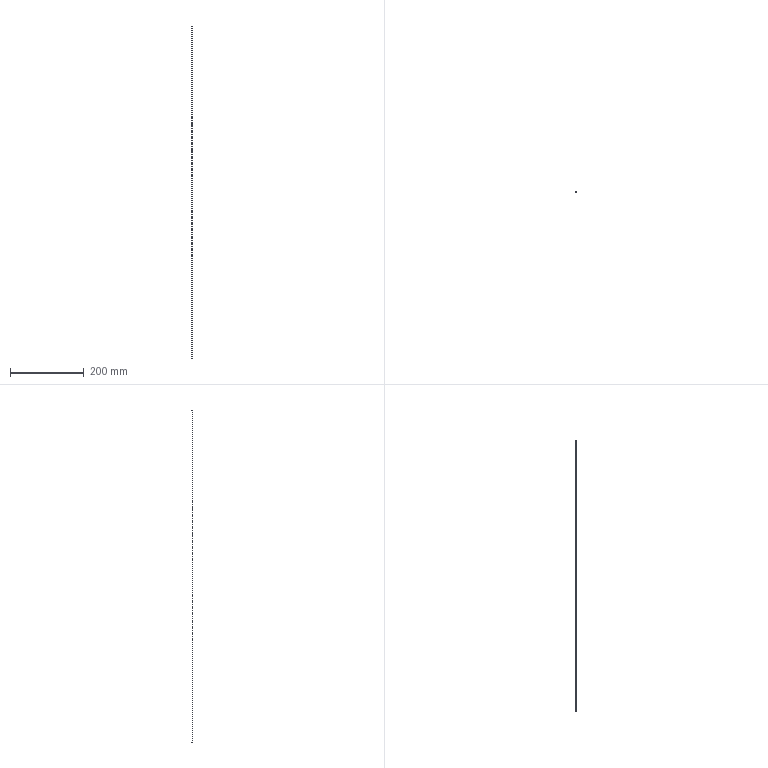Part | NX | 1 solid | 3 faces | box 2 x 2 x 900 mm | volume 2827 mm3 | plane 2 | cylinder 1 | commonest cylinder face diameters 2 x1
STEP:
#1=CARTESIAN_POINT('',(1.,0.,960.));
#2=VERTEX_POINT('',#1);
#3=CARTESIAN_POINT('',(0.,0.,960.));
#4=DIRECTION('',(0.,0.,1.));
#5=DIRECTION('',(1.,0.,0.));
#6=AXIS2_PLACEMENT_3D('',#3,#4,#5);
#7=CIRCLE('',#6,1.);
#8=EDGE_CURVE('',#2,#2,#7,.T.);
#9=ORIENTED_EDGE('',*,*,#8,.F.);
#10=EDGE_LOOP('',(#9));
#11=FACE_BOUND('',#10,.T.);
#12=CARTESIAN_POINT('',(1.,0.,60.));
#13=VERTEX_POINT('',#12);
#14=CARTESIAN_POINT('',(0.,0.,60.));
#15=DIRECTION('',(0.,0.,1.));
#16=DIRECTION('',(1.,0.,0.));
#17=AXIS2_PLACEMENT_3D('',#14,#15,#16);
#18=CIRCLE('',#17,1.);
#19=EDGE_CURVE('',#13,#13,#18,.T.);
#20=ORIENTED_EDGE('',*,*,#19,.T.);
#21=EDGE_LOOP('',(#20));
#22=FACE_BOUND('',#21,.T.);
#23=CARTESIAN_POINT('',(0.,0.,960.));
#24=DIRECTION('',(0.,0.,-1.));
#25=DIRECTION('',(-1.,0.,0.));
#26=AXIS2_PLACEMENT_3D('',#23,#24,#25);
#27=CYLINDRICAL_SURFACE('',#26,1.);
#28=ADVANCED_FACE('',(#11,#22),#27,.T.);
#29=ORIENTED_EDGE('',*,*,#8,.T.);
#30=EDGE_LOOP('',(#29));
#31=FACE_BOUND('',#30,.T.);
#32=CARTESIAN_POINT('',(0.,0.,960.));
#33=DIRECTION('',(0.,0.,1.));
#34=DIRECTION('',(1.,0.,0.));
#35=AXIS2_PLACEMENT_3D('',#32,#33,#34);
#36=PLANE('',#35);
#37=ADVANCED_FACE('',(#31),#36,.T.);
#38=ORIENTED_EDGE('',*,*,#19,.F.);
#39=EDGE_LOOP('',(#38));
#40=FACE_BOUND('',#39,.T.);
#41=CARTESIAN_POINT('',(0.,0.,60.));
#42=DIRECTION('',(0.,0.,1.));
#43=DIRECTION('',(1.,0.,0.));
#44=AXIS2_PLACEMENT_3D('',#41,#42,#43);
#45=PLANE('',#44);
#46=ADVANCED_FACE('',(#40),#45,.F.);
#47=CLOSED_SHELL('',(#28,#37,#46));
#48=MANIFOLD_SOLID_BREP('',#47);
#49=(LENGTH_UNIT()NAMED_UNIT(*)SI_UNIT(.MILLI.,.METRE.));
#50=UNCERTAINTY_MEASURE_WITH_UNIT(LENGTH_MEASURE(0.00001),#49,'','');
#51=(NAMED_UNIT(*)PLANE_ANGLE_UNIT()SI_UNIT($,.RADIAN.));
#52=(NAMED_UNIT(*)SI_UNIT($,.STERADIAN.)SOLID_ANGLE_UNIT());
#53=(GEOMETRIC_REPRESENTATION_CONTEXT(3)GLOBAL_UNCERTAINTY_ASSIGNED_CONTEXT((#50))GLOBAL_UNIT_ASSIGNED_CONTEXT((#49,#51,#52))REPRESENTATION_CONTEXT('',''));
#54=ADVANCED_BREP_SHAPE_REPRESENTATION('',(#48),#53);